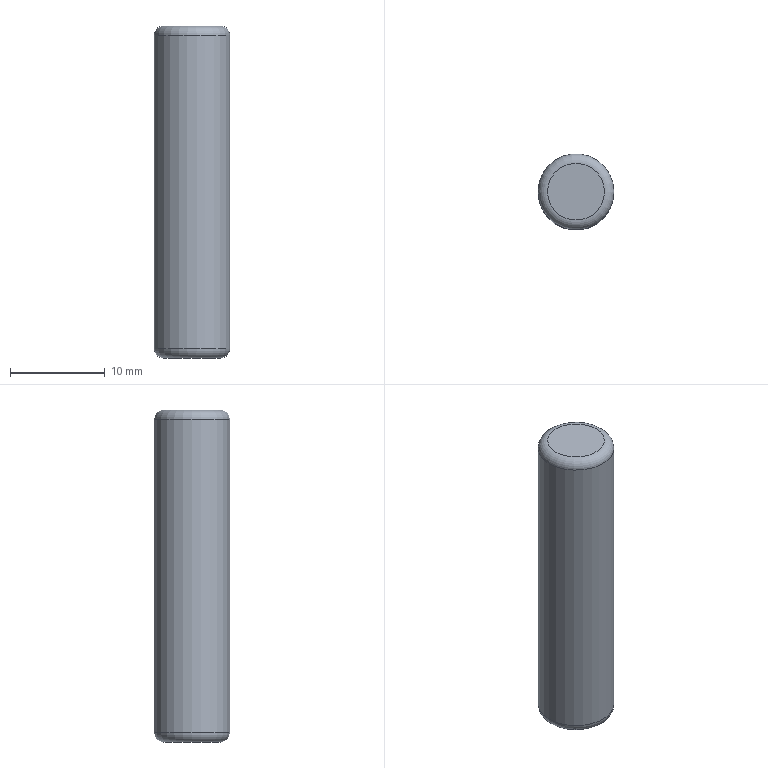Part | STEP file | 200 mesh_id702_x | 1 solid | 5 faces | box 8 x 8 x 35 mm | volume 1749 mm3 | plane 2 | torus 2 | cylinder 1 | commonest cylinder face diameters 8 x1
STEP:
#1=CARTESIAN_POINT('',(-16647.884,-4140.769,25.));
#2=VERTEX_POINT('',#1);
#3=CARTESIAN_POINT('',(-16650.884,-4140.769,25.));
#4=DIRECTION('',(0.,0.,1.));
#5=DIRECTION('',(1.,0.,0.));
#6=AXIS2_PLACEMENT_3D('',#3,#4,#5);
#7=CIRCLE('',#6,3.);
#8=EDGE_CURVE('',#2,#2,#7,.T.);
#9=ORIENTED_EDGE('',*,*,#8,.T.);
#10=EDGE_LOOP('',(#9));
#11=FACE_OUTER_BOUND('',#10,.T.);
#12=CARTESIAN_POINT('',(-16650.884,-4140.769,25.));
#13=DIRECTION('',(0.,0.,1.));
#14=DIRECTION('',(1.,0.,0.));
#15=AXIS2_PLACEMENT_3D('',#12,#13,#14);
#16=PLANE('',#15);
#17=ADVANCED_FACE('',(#11),#16,.T.);
#18=CARTESIAN_POINT('',(-16653.884,-4140.769,-10.));
#19=VERTEX_POINT('',#18);
#20=CARTESIAN_POINT('',(-16650.884,-4140.769,-10.));
#21=DIRECTION('',(0.,0.,-1.));
#22=DIRECTION('',(-1.,0.,0.));
#23=AXIS2_PLACEMENT_3D('',#20,#21,#22);
#24=CIRCLE('',#23,3.);
#25=EDGE_CURVE('',#19,#19,#24,.T.);
#26=ORIENTED_EDGE('',*,*,#25,.T.);
#27=EDGE_LOOP('',(#26));
#28=FACE_OUTER_BOUND('',#27,.T.);
#29=CARTESIAN_POINT('',(-16650.884,-4140.769,-10.));
#30=DIRECTION('',(0.,0.,-1.));
#31=DIRECTION('',(-1.,0.,0.));
#32=AXIS2_PLACEMENT_3D('',#29,#30,#31);
#33=PLANE('',#32);
#34=ADVANCED_FACE('',(#28),#33,.T.);
#35=CARTESIAN_POINT('',(-16654.884,-4140.769,-9.));
#36=VERTEX_POINT('',#35);
#37=CARTESIAN_POINT('',(-16650.884,-4140.769,-9.));
#38=DIRECTION('',(0.,0.,1.));
#39=DIRECTION('',(-1.,0.,0.));
#40=AXIS2_PLACEMENT_3D('',#37,#38,#39);
#41=CIRCLE('',#40,4.);
#42=EDGE_CURVE('',#36,#36,#41,.T.);
#43=ORIENTED_EDGE('',*,*,#42,.T.);
#44=EDGE_LOOP('',(#43));
#45=FACE_BOUND('',#44,.T.);
#46=CARTESIAN_POINT('',(-16646.884,-4140.769,24.));
#47=VERTEX_POINT('',#46);
#48=CARTESIAN_POINT('',(-16650.884,-4140.769,24.));
#49=DIRECTION('',(0.,0.,-1.));
#50=DIRECTION('',(1.,0.,0.));
#51=AXIS2_PLACEMENT_3D('',#48,#49,#50);
#52=CIRCLE('',#51,4.);
#53=EDGE_CURVE('',#47,#47,#52,.T.);
#54=ORIENTED_EDGE('',*,*,#53,.T.);
#55=EDGE_LOOP('',(#54));
#56=FACE_BOUND('',#55,.T.);
#57=CARTESIAN_POINT('',(-16650.884,-4140.769,0.));
#58=DIRECTION('',(0.,0.,1.));
#59=DIRECTION('',(1.,0.,0.));
#60=AXIS2_PLACEMENT_3D('',#57,#58,#59);
#61=CYLINDRICAL_SURFACE('',#60,4.);
#62=ADVANCED_FACE('',(#45,#56),#61,.T.);
#63=ORIENTED_EDGE('',*,*,#25,.F.);
#64=EDGE_LOOP('',(#63));
#65=FACE_BOUND('',#64,.T.);
#66=ORIENTED_EDGE('',*,*,#42,.F.);
#67=EDGE_LOOP('',(#66));
#68=FACE_BOUND('',#67,.T.);
#69=CARTESIAN_POINT('',(-16650.884,-4140.769,-9.));
#70=DIRECTION('',(0.,0.,-1.));
#71=DIRECTION('',(-1.,0.,0.));
#72=AXIS2_PLACEMENT_3D('',#69,#70,#71);
#73=TOROIDAL_SURFACE('',#72,3.,1.);
#74=ADVANCED_FACE('',(#65,#68),#73,.T.);
#75=ORIENTED_EDGE('',*,*,#8,.F.);
#76=EDGE_LOOP('',(#75));
#77=FACE_BOUND('',#76,.T.);
#78=ORIENTED_EDGE('',*,*,#53,.F.);
#79=EDGE_LOOP('',(#78));
#80=FACE_BOUND('',#79,.T.);
#81=CARTESIAN_POINT('',(-16650.884,-4140.769,24.));
#82=DIRECTION('',(0.,0.,1.));
#83=DIRECTION('',(1.,0.,0.));
#84=AXIS2_PLACEMENT_3D('',#81,#82,#83);
#85=TOROIDAL_SURFACE('',#84,3.,1.);
#86=ADVANCED_FACE('',(#77,#80),#85,.T.);
#87=CLOSED_SHELL('',(#17,#34,#62,#74,#86));
#88=MANIFOLD_SOLID_BREP('',#87);
#89=(LENGTH_UNIT()NAMED_UNIT(*)SI_UNIT(.MILLI.,.METRE.));
#90=UNCERTAINTY_MEASURE_WITH_UNIT(LENGTH_MEASURE(0.00002),#89,'','');
#91=(NAMED_UNIT(*)PLANE_ANGLE_UNIT()SI_UNIT($,.RADIAN.));
#92=PLANE_ANGLE_MEASURE_WITH_UNIT(PLANE_ANGLE_MEASURE(0.01745),#91);
#93=DIMENSIONAL_EXPONENTS(0.,0.,0.,0.,0.,0.,0.);
#94=(CONVERSION_BASED_UNIT('DEGREE',#92)NAMED_UNIT(#93)PLANE_ANGLE_UNIT());
#95=(NAMED_UNIT(*)SI_UNIT($,.STERADIAN.)SOLID_ANGLE_UNIT());
#96=(GEOMETRIC_REPRESENTATION_CONTEXT(3)GLOBAL_UNCERTAINTY_ASSIGNED_CONTEXT((#90))GLOBAL_UNIT_ASSIGNED_CONTEXT((#89,#94,#95))REPRESENTATION_CONTEXT('',''));
#97=ADVANCED_BREP_SHAPE_REPRESENTATION('',(#88),#96);